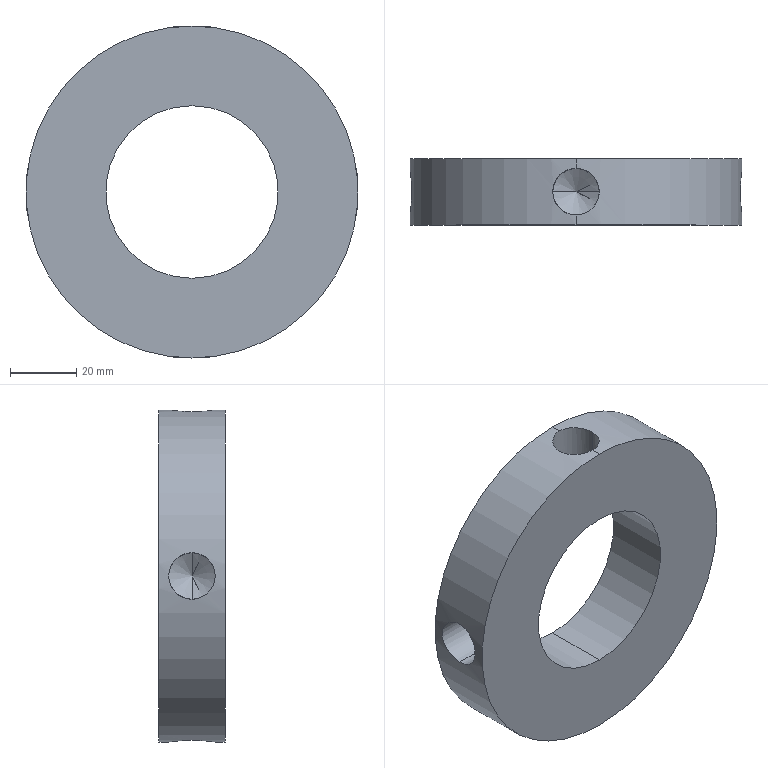Part | SolidWorks | features HoleWzd 2, 3DProfileFeature 1, CirPattern 1, Extrusion 1 | 1 solid | 22 faces | box 100 x 20 x 100 mm | volume 104092 mm3 | cylinder 12 | cone 8 | plane 2 | commonest cylinder face diameters 14 x8 52 x2 100 x2
STEP:
#1=CARTESIAN_POINT('',(-30.,10.,0.));
#2=VERTEX_POINT('',#1);
#3=CARTESIAN_POINT('',(-34.206,10.,7.));
#4=VERTEX_POINT('',#3);
#5=CARTESIAN_POINT('',(-34.206,10.,7.));
#6=DIRECTION('',(-0.515,0.,0.8572));
#7=VECTOR('',#6,1000.);
#8=LINE('',#5,#7);
#9=EDGE_CURVE('',#2,#4,#8,.T.);
#10=ORIENTED_EDGE('',*,*,#9,.F.);
#11=CARTESIAN_POINT('',(-34.206,10.,-7.));
#12=VERTEX_POINT('',#11);
#13=CARTESIAN_POINT('',(-34.206,10.,-7.));
#14=DIRECTION('',(-0.515,0.,-0.8572));
#15=VECTOR('',#14,1000.);
#16=LINE('',#13,#15);
#17=EDGE_CURVE('',#2,#12,#16,.T.);
#18=ORIENTED_EDGE('',*,*,#17,.T.);
#19=CARTESIAN_POINT('',(-34.206,10.,0.));
#20=DIRECTION('',(-1.,0.,0.));
#21=DIRECTION('',(0.,0.,1.));
#22=AXIS2_PLACEMENT_3D('',#19,#20,#21);
#23=CIRCLE('',#22,7.);
#24=EDGE_CURVE('',#12,#4,#23,.T.);
#25=ORIENTED_EDGE('',*,*,#24,.T.);
#26=EDGE_LOOP('',(#10,#18,#25));
#27=FACE_OUTER_BOUND('',#26,.T.);
#28=CARTESIAN_POINT('',(-34.206,10.,0.));
#29=DIRECTION('',(-1.,0.,0.));
#30=DIRECTION('',(0.,0.,1.));
#31=AXIS2_PLACEMENT_3D('',#28,#29,#30);
#32=CONICAL_SURFACE('',#31,7.,1.03);
#33=ADVANCED_FACE('',(#27),#32,.F.);
#34=ORIENTED_EDGE('',*,*,#24,.F.);
#35=CARTESIAN_POINT('',(-49.508,10.,-7.));
#36=VERTEX_POINT('',#35);
#37=CARTESIAN_POINT('',(-50.,10.,-7.));
#38=DIRECTION('',(-1.,0.,0.));
#39=VECTOR('',#38,1000.);
#40=LINE('',#37,#39);
#41=EDGE_CURVE('',#12,#36,#40,.T.);
#42=ORIENTED_EDGE('',*,*,#41,.T.);
#43=CARTESIAN_POINT('',(-49.508,10.,7.));
#44=VERTEX_POINT('',#43);
#45=CARTESIAN_POINT('',(-49.508,10.,7.));
#46=CARTESIAN_POINT('',(-49.508,9.537,7.));
#47=CARTESIAN_POINT('',(-49.514,9.082,6.954));
#48=CARTESIAN_POINT('',(-49.533,8.41,6.821));
#49=CARTESIAN_POINT('',(-49.54,8.188,6.765));
#50=CARTESIAN_POINT('',(-49.558,7.748,6.632));
#51=CARTESIAN_POINT('',(-49.569,7.529,6.554));
#52=CARTESIAN_POINT('',(-49.603,6.894,6.29));
#53=CARTESIAN_POINT('',(-49.63,6.492,6.075));
#54=CARTESIAN_POINT('',(-49.69,5.731,5.567));
#55=CARTESIAN_POINT('',(-49.722,5.372,5.271));
#56=CARTESIAN_POINT('',(-49.787,4.727,4.626));
#57=CARTESIAN_POINT('',(-49.818,4.437,4.274));
#58=CARTESIAN_POINT('',(-49.863,4.053,3.7));
#59=CARTESIAN_POINT('',(-49.878,3.935,3.502));
#60=CARTESIAN_POINT('',(-49.904,3.719,3.098));
#61=CARTESIAN_POINT('',(-49.929,3.524,2.686));
#62=CARTESIAN_POINT('',(-49.95,3.369,2.256));
#63=CARTESIAN_POINT('',(-49.967,3.236,1.817));
#64=CARTESIAN_POINT('',(-49.975,3.18,1.592));
#65=CARTESIAN_POINT('',(-49.994,3.045,0.9144));
#66=CARTESIAN_POINT('',(-50.,3.,0.4598));
#67=CARTESIAN_POINT('',(-50.,3.,-0.4546));
#68=CARTESIAN_POINT('',(-49.994,3.046,-0.9191));
#69=CARTESIAN_POINT('',(-49.969,3.225,-1.817));
#70=CARTESIAN_POINT('',(-49.951,3.357,-2.254));
#71=CARTESIAN_POINT('',(-49.917,3.62,-2.89));
#72=CARTESIAN_POINT('',(-49.904,3.72,-3.1));
#73=CARTESIAN_POINT('',(-49.877,3.936,-3.505));
#74=CARTESIAN_POINT('',(-49.863,4.054,-3.701));
#75=CARTESIAN_POINT('',(-49.819,4.434,-4.269));
#76=CARTESIAN_POINT('',(-49.787,4.724,-4.623));
#77=CARTESIAN_POINT('',(-49.722,5.376,-5.276));
#78=CARTESIAN_POINT('',(-49.69,5.729,-5.565));
#79=CARTESIAN_POINT('',(-49.645,6.298,-5.945));
#80=CARTESIAN_POINT('',(-49.631,6.493,-6.063));
#81=CARTESIAN_POINT('',(-49.604,6.899,-6.28));
#82=CARTESIAN_POINT('',(-49.592,7.108,-6.379));
#83=CARTESIAN_POINT('',(-49.557,7.744,-6.642));
#84=CARTESIAN_POINT('',(-49.539,8.18,-6.775));
#85=CARTESIAN_POINT('',(-49.514,9.078,-6.954));
#86=CARTESIAN_POINT('',(-49.508,9.543,-7.));
#87=CARTESIAN_POINT('',(-49.508,10.,-7.));
#88=B_SPLINE_CURVE_WITH_KNOTS('',3,(#45,#46,#47,#48,#49,#50,#51,#52,#53,#54,#55,#56,#57,#58,#59,#60,#61,#62,#63,#64,#65,#66,#67,#68,#69,#70,#71,#72,#73,#74,#75,#76,#77,#78,#79,#80,#81,#82,#83,#84,#85,#86,#87),.UNSPECIFIED.,.F.,.F.,(4,2,2,2,2,2,2,2,1,2,2,2,2,2,2,2,2,2,2,2,2,4),(0.,0.00137,0.002054,0.002739,0.004109,0.005478,0.006848,0.007532,0.008217,0.008902,0.009587,0.01096,0.01233,0.0137,0.01438,0.01506,0.01643,0.0178,0.01849,0.01917,0.02054,0.02191),.UNSPECIFIED.);
#89=EDGE_CURVE('',#44,#36,#88,.T.);
#90=ORIENTED_EDGE('',*,*,#89,.F.);
#91=CARTESIAN_POINT('',(-50.,10.,7.));
#92=DIRECTION('',(-1.,0.,0.));
#93=VECTOR('',#92,1000.);
#94=LINE('',#91,#93);
#95=EDGE_CURVE('',#4,#44,#94,.T.);
#96=ORIENTED_EDGE('',*,*,#95,.F.);
#97=EDGE_LOOP('',(#34,#42,#90,#96));
#98=FACE_OUTER_BOUND('',#97,.T.);
#99=CARTESIAN_POINT('',(-50.,10.,0.));
#100=DIRECTION('',(-1.,0.,0.));
#101=DIRECTION('',(0.,0.,1.));
#102=AXIS2_PLACEMENT_3D('',#99,#100,#101);
#103=CYLINDRICAL_SURFACE('',#102,7.);
#104=ADVANCED_FACE('',(#98),#103,.F.);
#105=CARTESIAN_POINT('',(0.,10.,-30.));
#106=VERTEX_POINT('',#105);
#107=CARTESIAN_POINT('',(-7.,10.,-34.206));
#108=VERTEX_POINT('',#107);
#109=CARTESIAN_POINT('',(-7.,10.,-34.206));
#110=DIRECTION('',(-0.8572,0.,-0.515));
#111=VECTOR('',#110,1000.);
#112=LINE('',#109,#111);
#113=EDGE_CURVE('',#106,#108,#112,.T.);
#114=ORIENTED_EDGE('',*,*,#113,.F.);
#115=CARTESIAN_POINT('',(7.,10.,-34.206));
#116=VERTEX_POINT('',#115);
#117=CARTESIAN_POINT('',(7.,10.,-34.206));
#118=DIRECTION('',(0.8572,0.,-0.515));
#119=VECTOR('',#118,1000.);
#120=LINE('',#117,#119);
#121=EDGE_CURVE('',#106,#116,#120,.T.);
#122=ORIENTED_EDGE('',*,*,#121,.T.);
#123=CARTESIAN_POINT('',(0.,10.,-34.206));
#124=DIRECTION('',(0.,0.,-1.));
#125=DIRECTION('',(-1.,0.,0.));
#126=AXIS2_PLACEMENT_3D('',#123,#124,#125);
#127=CIRCLE('',#126,7.);
#128=EDGE_CURVE('',#116,#108,#127,.T.);
#129=ORIENTED_EDGE('',*,*,#128,.T.);
#130=EDGE_LOOP('',(#114,#122,#129));
#131=FACE_OUTER_BOUND('',#130,.T.);
#132=CARTESIAN_POINT('',(0.,10.,-34.206));
#133=DIRECTION('',(0.,0.,-1.));
#134=DIRECTION('',(-1.,0.,0.));
#135=AXIS2_PLACEMENT_3D('',#132,#133,#134);
#136=CONICAL_SURFACE('',#135,7.,1.03);
#137=ADVANCED_FACE('',(#131),#136,.F.);
#138=ORIENTED_EDGE('',*,*,#128,.F.);
#139=CARTESIAN_POINT('',(7.,10.,-49.508));
#140=VERTEX_POINT('',#139);
#141=CARTESIAN_POINT('',(7.,10.,-50.));
#142=DIRECTION('',(0.,0.,-1.));
#143=VECTOR('',#142,1000.);
#144=LINE('',#141,#143);
#145=EDGE_CURVE('',#116,#140,#144,.T.);
#146=ORIENTED_EDGE('',*,*,#145,.T.);
#147=CARTESIAN_POINT('',(0.,3.,-50.));
#148=VERTEX_POINT('',#147);
#149=CARTESIAN_POINT('',(0.,3.,-50.));
#150=CARTESIAN_POINT('',(0.4572,3.,-50.));
#151=CARTESIAN_POINT('',(0.9121,3.044,-49.994));
#152=CARTESIAN_POINT('',(1.591,3.179,-49.975));
#153=CARTESIAN_POINT('',(1.815,3.236,-49.968));
#154=CARTESIAN_POINT('',(2.254,3.369,-49.95));
#155=CARTESIAN_POINT('',(2.684,3.523,-49.929));
#156=CARTESIAN_POINT('',(3.097,3.718,-49.904));
#157=CARTESIAN_POINT('',(3.501,3.934,-49.878));
#158=CARTESIAN_POINT('',(3.7,4.053,-49.863));
#159=CARTESIAN_POINT('',(4.273,4.437,-49.819));
#160=CARTESIAN_POINT('',(4.625,4.726,-49.787));
#161=CARTESIAN_POINT('',(5.271,5.371,-49.722));
#162=CARTESIAN_POINT('',(5.567,5.731,-49.69));
#163=CARTESIAN_POINT('',(6.074,6.491,-49.63));
#164=CARTESIAN_POINT('',(6.289,6.893,-49.603));
#165=CARTESIAN_POINT('',(6.553,7.529,-49.569));
#166=CARTESIAN_POINT('',(6.632,7.748,-49.558));
#167=CARTESIAN_POINT('',(6.765,8.188,-49.54));
#168=CARTESIAN_POINT('',(6.821,8.409,-49.533));
#169=CARTESIAN_POINT('',(6.954,9.081,-49.514));
#170=CARTESIAN_POINT('',(7.,9.537,-49.508));
#171=CARTESIAN_POINT('',(7.,10.,-49.508));
#172=B_SPLINE_CURVE_WITH_KNOTS('',3,(#149,#150,#151,#152,#153,#154,#155,#156,#157,#158,#159,#160,#161,#162,#163,#164,#165,#166,#167,#168,#169,#170,#171),.UNSPECIFIED.,.F.,.F.,(4,2,2,1,2,2,2,2,2,2,2,4),(0.02191,0.02328,0.02397,0.02465,0.02534,0.02602,0.02739,0.02876,0.03013,0.03082,0.0315,0.03287),.UNSPECIFIED.);
#173=EDGE_CURVE('',#148,#140,#172,.T.);
#174=ORIENTED_EDGE('',*,*,#173,.F.);
#175=CARTESIAN_POINT('',(-7.,10.,-49.508));
#176=VERTEX_POINT('',#175);
#177=CARTESIAN_POINT('',(-7.,10.,-49.508));
#178=CARTESIAN_POINT('',(-7.,9.543,-49.508));
#179=CARTESIAN_POINT('',(-6.954,9.079,-49.514));
#180=CARTESIAN_POINT('',(-6.775,8.181,-49.539));
#181=CARTESIAN_POINT('',(-6.642,7.744,-49.557));
#182=CARTESIAN_POINT('',(-6.379,7.108,-49.592));
#183=CARTESIAN_POINT('',(-6.28,6.898,-49.604));
#184=CARTESIAN_POINT('',(-6.063,6.494,-49.631));
#185=CARTESIAN_POINT('',(-5.945,6.298,-49.645));
#186=CARTESIAN_POINT('',(-5.565,5.73,-49.69));
#187=CARTESIAN_POINT('',(-5.275,5.376,-49.722));
#188=CARTESIAN_POINT('',(-4.623,4.723,-49.787));
#189=CARTESIAN_POINT('',(-4.27,4.434,-49.819));
#190=CARTESIAN_POINT('',(-3.702,4.054,-49.863));
#191=CARTESIAN_POINT('',(-3.506,3.937,-49.877));
#192=CARTESIAN_POINT('',(-3.101,3.72,-49.904));
#193=CARTESIAN_POINT('',(-2.891,3.621,-49.917));
#194=CARTESIAN_POINT('',(-2.256,3.358,-49.951));
#195=CARTESIAN_POINT('',(-1.819,3.225,-49.969));
#196=CARTESIAN_POINT('',(-0.9213,3.046,-49.994));
#197=CARTESIAN_POINT('',(-0.457,3.,-50.));
#198=CARTESIAN_POINT('',(0.,3.,-50.));
#199=B_SPLINE_CURVE_WITH_KNOTS('',3,(#177,#178,#179,#180,#181,#182,#183,#184,#185,#186,#187,#188,#189,#190,#191,#192,#193,#194,#195,#196,#197,#198),.UNSPECIFIED.,.F.,.F.,(4,2,2,2,2,2,2,2,2,2,4),(0.01096,0.01233,0.0137,0.01438,0.01507,0.01644,0.0178,0.01849,0.01917,0.02054,0.02191),.UNSPECIFIED.);
#200=EDGE_CURVE('',#176,#148,#199,.T.);
#201=ORIENTED_EDGE('',*,*,#200,.F.);
#202=CARTESIAN_POINT('',(-7.,10.,-50.));
#203=DIRECTION('',(0.,0.,-1.));
#204=VECTOR('',#203,1000.);
#205=LINE('',#202,#204);
#206=EDGE_CURVE('',#108,#176,#205,.T.);
#207=ORIENTED_EDGE('',*,*,#206,.F.);
#208=EDGE_LOOP('',(#138,#146,#174,#201,#207));
#209=FACE_OUTER_BOUND('',#208,.T.);
#210=CARTESIAN_POINT('',(0.,10.,-50.));
#211=DIRECTION('',(0.,0.,-1.));
#212=DIRECTION('',(-1.,0.,0.));
#213=AXIS2_PLACEMENT_3D('',#210,#211,#212);
#214=CYLINDRICAL_SURFACE('',#213,7.);
#215=ADVANCED_FACE('',(#209),#214,.F.);
#216=CARTESIAN_POINT('',(30.,10.,0.));
#217=VERTEX_POINT('',#216);
#218=CARTESIAN_POINT('',(34.206,10.,-7.));
#219=VERTEX_POINT('',#218);
#220=CARTESIAN_POINT('',(34.206,10.,-7.));
#221=DIRECTION('',(0.515,0.,-0.8572));
#222=VECTOR('',#221,1000.);
#223=LINE('',#220,#222);
#224=EDGE_CURVE('',#217,#219,#223,.T.);
#225=ORIENTED_EDGE('',*,*,#224,.F.);
#226=CARTESIAN_POINT('',(34.206,10.,7.));
#227=VERTEX_POINT('',#226);
#228=CARTESIAN_POINT('',(34.206,10.,7.));
#229=DIRECTION('',(0.515,0.,0.8572));
#230=VECTOR('',#229,1000.);
#231=LINE('',#228,#230);
#232=EDGE_CURVE('',#217,#227,#231,.T.);
#233=ORIENTED_EDGE('',*,*,#232,.T.);
#234=CARTESIAN_POINT('',(34.206,10.,0.));
#235=DIRECTION('',(1.,0.,0.));
#236=DIRECTION('',(0.,0.,-1.));
#237=AXIS2_PLACEMENT_3D('',#234,#235,#236);
#238=CIRCLE('',#237,7.);
#239=EDGE_CURVE('',#227,#219,#238,.T.);
#240=ORIENTED_EDGE('',*,*,#239,.T.);
#241=EDGE_LOOP('',(#225,#233,#240));
#242=FACE_OUTER_BOUND('',#241,.T.);
#243=CARTESIAN_POINT('',(34.206,10.,0.));
#244=DIRECTION('',(1.,0.,0.));
#245=DIRECTION('',(0.,0.,-1.));
#246=AXIS2_PLACEMENT_3D('',#243,#244,#245);
#247=CONICAL_SURFACE('',#246,7.,1.03);
#248=ADVANCED_FACE('',(#242),#247,.F.);
#249=ORIENTED_EDGE('',*,*,#239,.F.);
#250=CARTESIAN_POINT('',(49.508,10.,7.));
#251=VERTEX_POINT('',#250);
#252=CARTESIAN_POINT('',(50.,10.,7.));
#253=DIRECTION('',(1.,0.,0.));
#254=VECTOR('',#253,1000.);
#255=LINE('',#252,#254);
#256=EDGE_CURVE('',#227,#251,#255,.T.);
#257=ORIENTED_EDGE('',*,*,#256,.T.);
#258=CARTESIAN_POINT('',(49.508,10.,-7.));
#259=VERTEX_POINT('',#258);
#260=CARTESIAN_POINT('',(49.508,10.,-7.));
#261=CARTESIAN_POINT('',(49.508,9.537,-7.));
#262=CARTESIAN_POINT('',(49.514,9.082,-6.954));
#263=CARTESIAN_POINT('',(49.533,8.41,-6.821));
#264=CARTESIAN_POINT('',(49.54,8.188,-6.765));
#265=CARTESIAN_POINT('',(49.558,7.748,-6.632));
#266=CARTESIAN_POINT('',(49.569,7.529,-6.554));
#267=CARTESIAN_POINT('',(49.603,6.894,-6.29));
#268=CARTESIAN_POINT('',(49.63,6.492,-6.075));
#269=CARTESIAN_POINT('',(49.69,5.731,-5.567));
#270=CARTESIAN_POINT('',(49.722,5.372,-5.271));
#271=CARTESIAN_POINT('',(49.787,4.727,-4.626));
#272=CARTESIAN_POINT('',(49.818,4.437,-4.274));
#273=CARTESIAN_POINT('',(49.863,4.053,-3.7));
#274=CARTESIAN_POINT('',(49.878,3.935,-3.502));
#275=CARTESIAN_POINT('',(49.904,3.719,-3.098));
#276=CARTESIAN_POINT('',(49.929,3.524,-2.686));
#277=CARTESIAN_POINT('',(49.95,3.369,-2.256));
#278=CARTESIAN_POINT('',(49.967,3.236,-1.817));
#279=CARTESIAN_POINT('',(49.975,3.18,-1.592));
#280=CARTESIAN_POINT('',(49.994,3.045,-0.9144));
#281=CARTESIAN_POINT('',(50.,3.,-0.4598));
#282=CARTESIAN_POINT('',(50.,3.,0.4546));
#283=CARTESIAN_POINT('',(49.994,3.046,0.9191));
#284=CARTESIAN_POINT('',(49.969,3.225,1.817));
#285=CARTESIAN_POINT('',(49.951,3.357,2.254));
#286=CARTESIAN_POINT('',(49.917,3.62,2.89));
#287=CARTESIAN_POINT('',(49.904,3.72,3.1));
#288=CARTESIAN_POINT('',(49.877,3.936,3.505));
#289=CARTESIAN_POINT('',(49.863,4.054,3.701));
#290=CARTESIAN_POINT('',(49.819,4.434,4.269));
#291=CARTESIAN_POINT('',(49.787,4.724,4.623));
#292=CARTESIAN_POINT('',(49.722,5.376,5.276));
#293=CARTESIAN_POINT('',(49.69,5.729,5.565));
#294=CARTESIAN_POINT('',(49.645,6.298,5.945));
#295=CARTESIAN_POINT('',(49.631,6.493,6.063));
#296=CARTESIAN_POINT('',(49.604,6.899,6.28));
#297=CARTESIAN_POINT('',(49.592,7.108,6.379));
#298=CARTESIAN_POINT('',(49.557,7.744,6.642));
#299=CARTESIAN_POINT('',(49.539,8.18,6.775));
#300=CARTESIAN_POINT('',(49.514,9.078,6.954));
#301=CARTESIAN_POINT('',(49.508,9.543,7.));
#302=CARTESIAN_POINT('',(49.508,10.,7.));
#303=B_SPLINE_CURVE_WITH_KNOTS('',3,(#260,#261,#262,#263,#264,#265,#266,#267,#268,#269,#270,#271,#272,#273,#274,#275,#276,#277,#278,#279,#280,#281,#282,#283,#284,#285,#286,#287,#288,#289,#290,#291,#292,#293,#294,#295,#296,#297,#298,#299,#300,#301,#302),.UNSPECIFIED.,.F.,.F.,(4,2,2,2,2,2,2,2,1,2,2,2,2,2,2,2,2,2,2,2,2,4),(0.,0.00137,0.002054,0.002739,0.004109,0.005478,0.006848,0.007532,0.008217,0.008902,0.009587,0.01096,0.01233,0.0137,0.01438,0.01506,0.01643,0.0178,0.01849,0.01917,0.02054,0.02191),.UNSPECIFIED.);
#304=EDGE_CURVE('',#259,#251,#303,.T.);
#305=ORIENTED_EDGE('',*,*,#304,.F.);
#306=CARTESIAN_POINT('',(50.,10.,-7.));
#307=DIRECTION('',(1.,0.,0.));
#308=VECTOR('',#307,1000.);
#309=LINE('',#306,#308);
#310=EDGE_CURVE('',#219,#259,#309,.T.);
#311=ORIENTED_EDGE('',*,*,#310,.F.);
#312=EDGE_LOOP('',(#249,#257,#305,#311));
#313=FACE_OUTER_BOUND('',#312,.T.);
#314=CARTESIAN_POINT('',(50.,10.,0.));
#315=DIRECTION('',(1.,0.,0.));
#316=DIRECTION('',(0.,0.,-1.));
#317=AXIS2_PLACEMENT_3D('',#314,#315,#316);
#318=CYLINDRICAL_SURFACE('',#317,7.);
#319=ADVANCED_FACE('',(#313),#318,.F.);
#320=CARTESIAN_POINT('',(0.,10.,30.));
#321=VERTEX_POINT('',#320);
#322=CARTESIAN_POINT('',(7.,10.,34.206));
#323=VERTEX_POINT('',#322);
#324=CARTESIAN_POINT('',(7.,10.,34.206));
#325=DIRECTION('',(0.8572,0.,0.515));
#326=VECTOR('',#325,1000.);
#327=LINE('',#324,#326);
#328=EDGE_CURVE('',#321,#323,#327,.T.);
#329=ORIENTED_EDGE('',*,*,#328,.F.);
#330=CARTESIAN_POINT('',(-7.,10.,34.206));
#331=VERTEX_POINT('',#330);
#332=CARTESIAN_POINT('',(-7.,10.,34.206));
#333=DIRECTION('',(-0.8572,0.,0.515));
#334=VECTOR('',#333,1000.);
#335=LINE('',#332,#334);
#336=EDGE_CURVE('',#321,#331,#335,.T.);
#337=ORIENTED_EDGE('',*,*,#336,.T.);
#338=CARTESIAN_POINT('',(0.,10.,34.206));
#339=DIRECTION('',(0.,0.,1.));
#340=DIRECTION('',(1.,0.,0.));
#341=AXIS2_PLACEMENT_3D('',#338,#339,#340);
#342=CIRCLE('',#341,7.);
#343=EDGE_CURVE('',#331,#323,#342,.T.);
#344=ORIENTED_EDGE('',*,*,#343,.T.);
#345=EDGE_LOOP('',(#329,#337,#344));
#346=FACE_OUTER_BOUND('',#345,.T.);
#347=CARTESIAN_POINT('',(0.,10.,34.206));
#348=DIRECTION('',(0.,0.,1.));
#349=DIRECTION('',(1.,0.,0.));
#350=AXIS2_PLACEMENT_3D('',#347,#348,#349);
#351=CONICAL_SURFACE('',#350,7.,1.03);
#352=ADVANCED_FACE('',(#346),#351,.F.);
#353=ORIENTED_EDGE('',*,*,#343,.F.);
#354=CARTESIAN_POINT('',(-7.,10.,49.508));
#355=VERTEX_POINT('',#354);
#356=CARTESIAN_POINT('',(-7.,10.,50.));
#357=DIRECTION('',(0.,0.,1.));
#358=VECTOR('',#357,1000.);
#359=LINE('',#356,#358);
#360=EDGE_CURVE('',#331,#355,#359,.T.);
#361=ORIENTED_EDGE('',*,*,#360,.T.);
#362=CARTESIAN_POINT('',(0.,3.,50.));
#363=VERTEX_POINT('',#362);
#364=CARTESIAN_POINT('',(0.,3.,50.));
#365=CARTESIAN_POINT('',(-0.4571,3.,50.));
#366=CARTESIAN_POINT('',(-0.9214,3.046,49.994));
#367=CARTESIAN_POINT('',(-1.819,3.225,49.969));
#368=CARTESIAN_POINT('',(-2.256,3.358,49.951));
#369=CARTESIAN_POINT('',(-2.892,3.621,49.917));
#370=CARTESIAN_POINT('',(-3.102,3.72,49.904));
#371=CARTESIAN_POINT('',(-3.506,3.937,49.877));
#372=CARTESIAN_POINT('',(-3.702,4.055,49.863));
#373=CARTESIAN_POINT('',(-4.27,4.435,49.819));
#374=CARTESIAN_POINT('',(-4.624,4.725,49.787));
#375=CARTESIAN_POINT('',(-5.277,5.377,49.722));
#376=CARTESIAN_POINT('',(-5.566,5.73,49.69));
#377=CARTESIAN_POINT('',(-5.946,6.298,49.645));
#378=CARTESIAN_POINT('',(-6.063,6.494,49.631));
#379=CARTESIAN_POINT('',(-6.28,6.899,49.604));
#380=CARTESIAN_POINT('',(-6.379,7.109,49.591));
#381=CARTESIAN_POINT('',(-6.642,7.744,49.557));
#382=CARTESIAN_POINT('',(-6.775,8.181,49.539));
#383=CARTESIAN_POINT('',(-6.954,9.079,49.514));
#384=CARTESIAN_POINT('',(-7.,9.543,49.508));
#385=CARTESIAN_POINT('',(-7.,10.,49.508));
#386=B_SPLINE_CURVE_WITH_KNOTS('',3,(#364,#365,#366,#367,#368,#369,#370,#371,#372,#373,#374,#375,#376,#377,#378,#379,#380,#381,#382,#383,#384,#385),.UNSPECIFIED.,.F.,.F.,(4,2,2,2,2,2,2,2,2,2,4),(0.01096,0.01233,0.0137,0.01438,0.01507,0.01644,0.0178,0.01849,0.01917,0.02054,0.02191),.UNSPECIFIED.);
#387=EDGE_CURVE('',#363,#355,#386,.T.);
#388=ORIENTED_EDGE('',*,*,#387,.F.);
#389=CARTESIAN_POINT('',(7.,10.,49.508));
#390=VERTEX_POINT('',#389);
#391=CARTESIAN_POINT('',(7.,10.,49.508));
#392=CARTESIAN_POINT('',(7.,9.537,49.508));
#393=CARTESIAN_POINT('',(6.954,9.081,49.514));
#394=CARTESIAN_POINT('',(6.821,8.41,49.533));
#395=CARTESIAN_POINT('',(6.765,8.188,49.54));
#396=CARTESIAN_POINT('',(6.632,7.747,49.558));
#397=CARTESIAN_POINT('',(6.553,7.529,49.569));
#398=CARTESIAN_POINT('',(6.289,6.893,49.603));
#399=CARTESIAN_POINT('',(6.074,6.491,49.63));
#400=CARTESIAN_POINT('',(5.566,5.73,49.69));
#401=CARTESIAN_POINT('',(5.271,5.371,49.722));
#402=CARTESIAN_POINT('',(4.625,4.726,49.787));
#403=CARTESIAN_POINT('',(4.273,4.436,49.819));
#404=CARTESIAN_POINT('',(3.699,4.053,49.863));
#405=CARTESIAN_POINT('',(3.5,3.934,49.878));
#406=CARTESIAN_POINT('',(3.096,3.718,49.904));
#407=CARTESIAN_POINT('',(2.684,3.523,49.929));
#408=CARTESIAN_POINT('',(2.254,3.369,49.95));
#409=CARTESIAN_POINT('',(1.815,3.236,49.968));
#410=CARTESIAN_POINT('',(1.59,3.179,49.975));
#411=CARTESIAN_POINT('',(0.912,3.044,49.994));
#412=CARTESIAN_POINT('',(0.4573,3.,50.));
#413=CARTESIAN_POINT('',(0.,3.,50.));
#414=B_SPLINE_CURVE_WITH_KNOTS('',3,(#391,#392,#393,#394,#395,#396,#397,#398,#399,#400,#401,#402,#403,#404,#405,#406,#407,#408,#409,#410,#411,#412,#413),.UNSPECIFIED.,.F.,.F.,(4,2,2,2,2,2,2,2,1,2,2,4),(0.,0.00137,0.002055,0.00274,0.004109,0.005479,0.006849,0.007534,0.008219,0.008904,0.009589,0.01096),.UNSPECIFIED.);
#415=EDGE_CURVE('',#390,#363,#414,.T.);
#416=ORIENTED_EDGE('',*,*,#415,.F.);
#417=CARTESIAN_POINT('',(7.,10.,50.));
#418=DIRECTION('',(0.,0.,1.));
#419=VECTOR('',#418,1000.);
#420=LINE('',#417,#419);
#421=EDGE_CURVE('',#323,#390,#420,.T.);
#422=ORIENTED_EDGE('',*,*,#421,.F.);
#423=EDGE_LOOP('',(#353,#361,#388,#416,#422));
#424=FACE_OUTER_BOUND('',#423,.T.);
#425=CARTESIAN_POINT('',(0.,10.,50.));
#426=DIRECTION('',(0.,0.,1.));
#427=DIRECTION('',(1.,0.,0.));
#428=AXIS2_PLACEMENT_3D('',#425,#426,#427);
#429=CYLINDRICAL_SURFACE('',#428,7.);
#430=ADVANCED_FACE('',(#424),#429,.F.);
#431=CARTESIAN_POINT('',(0.,0.,-26.));
#432=VERTEX_POINT('',#431);
#433=CARTESIAN_POINT('',(0.,0.,26.));
#434=VERTEX_POINT('',#433);
#435=CARTESIAN_POINT('',(0.,0.,0.));
#436=DIRECTION('',(0.,1.,0.));
#437=DIRECTION('',(0.,0.,1.));
#438=AXIS2_PLACEMENT_3D('',#435,#436,#437);
#439=CIRCLE('',#438,26.);
#440=EDGE_CURVE('',#432,#434,#439,.T.);
#441=ORIENTED_EDGE('',*,*,#440,.F.);
#442=CARTESIAN_POINT('',(0.,20.,-26.));
#443=VERTEX_POINT('',#442);
#444=CARTESIAN_POINT('',(0.,20.,-26.));
#445=DIRECTION('',(0.,1.,0.));
#446=VECTOR('',#445,1000.);
#447=LINE('',#444,#446);
#448=EDGE_CURVE('',#432,#443,#447,.T.);
#449=ORIENTED_EDGE('',*,*,#448,.T.);
#450=CARTESIAN_POINT('',(0.,20.,26.));
#451=VERTEX_POINT('',#450);
#452=CARTESIAN_POINT('',(0.,20.,0.));
#453=DIRECTION('',(0.,1.,0.));
#454=DIRECTION('',(0.,0.,1.));
#455=AXIS2_PLACEMENT_3D('',#452,#453,#454);
#456=CIRCLE('',#455,26.);
#457=EDGE_CURVE('',#443,#451,#456,.T.);
#458=ORIENTED_EDGE('',*,*,#457,.T.);
#459=CARTESIAN_POINT('',(0.,20.,26.));
#460=DIRECTION('',(0.,1.,0.));
#461=VECTOR('',#460,1000.);
#462=LINE('',#459,#461);
#463=EDGE_CURVE('',#434,#451,#462,.T.);
#464=ORIENTED_EDGE('',*,*,#463,.F.);
#465=EDGE_LOOP('',(#441,#449,#458,#464));
#466=FACE_OUTER_BOUND('',#465,.T.);
#467=CARTESIAN_POINT('',(0.,20.,0.));
#468=DIRECTION('',(0.,1.,0.));
#469=DIRECTION('',(0.,0.,1.));
#470=AXIS2_PLACEMENT_3D('',#467,#468,#469);
#471=CYLINDRICAL_SURFACE('',#470,26.);
#472=ADVANCED_FACE('',(#466),#471,.F.);
#473=ORIENTED_EDGE('',*,*,#304,.T.);
#474=CARTESIAN_POINT('',(49.508,10.,7.));
#475=CARTESIAN_POINT('',(49.508,10.457,7.));
#476=CARTESIAN_POINT('',(49.514,10.912,6.956));
#477=CARTESIAN_POINT('',(49.533,11.59,6.821));
#478=CARTESIAN_POINT('',(49.54,11.815,6.765));
#479=CARTESIAN_POINT('',(49.558,12.253,6.631));
#480=CARTESIAN_POINT('',(49.579,12.683,6.478));
#481=CARTESIAN_POINT('',(49.604,13.095,6.283));
#482=CARTESIAN_POINT('',(49.631,13.5,6.067));
#483=CARTESIAN_POINT('',(49.645,13.698,5.948));
#484=CARTESIAN_POINT('',(49.69,14.272,5.565));
#485=CARTESIAN_POINT('',(49.722,14.624,5.275));
#486=CARTESIAN_POINT('',(49.786,15.269,4.631));
#487=CARTESIAN_POINT('',(49.819,15.565,4.271));
#488=CARTESIAN_POINT('',(49.878,16.073,3.512));
#489=CARTESIAN_POINT('',(49.905,16.288,3.11));
#490=CARTESIAN_POINT('',(49.939,16.552,2.474));
#491=CARTESIAN_POINT('',(49.95,16.631,2.256));
#492=CARTESIAN_POINT('',(49.967,16.764,1.816));
#493=CARTESIAN_POINT('',(49.975,16.82,1.594));
#494=CARTESIAN_POINT('',(49.993,16.954,0.9233));
#495=CARTESIAN_POINT('',(50.,17.,0.4674));
#496=CARTESIAN_POINT('',(50.,17.,-0.458));
#497=CARTESIAN_POINT('',(49.994,16.955,-0.913));
#498=CARTESIAN_POINT('',(49.975,16.822,-1.585));
#499=CARTESIAN_POINT('',(49.968,16.767,-1.807));
#500=CARTESIAN_POINT('',(49.95,16.633,-2.247));
#501=CARTESIAN_POINT('',(49.94,16.555,-2.466));
#502=CARTESIAN_POINT('',(49.906,16.292,-3.101));
#503=CARTESIAN_POINT('',(49.879,16.078,-3.503));
#504=CARTESIAN_POINT('',(49.834,15.697,-4.074));
#505=CARTESIAN_POINT('',(49.819,15.559,-4.26));
#506=CARTESIAN_POINT('',(49.787,15.268,-4.616));
#507=CARTESIAN_POINT('',(49.771,15.114,-4.785));
#508=CARTESIAN_POINT('',(49.723,14.631,-5.269));
#509=CARTESIAN_POINT('',(49.691,14.279,-5.559));
#510=CARTESIAN_POINT('',(49.646,13.705,-5.943));
#511=CARTESIAN_POINT('',(49.631,13.507,-6.062));
#512=CARTESIAN_POINT('',(49.604,13.104,-6.278));
#513=CARTESIAN_POINT('',(49.579,12.692,-6.474));
#514=CARTESIAN_POINT('',(49.559,12.262,-6.628));
#515=CARTESIAN_POINT('',(49.541,11.824,-6.762));
#516=CARTESIAN_POINT('',(49.533,11.599,-6.819));
#517=CARTESIAN_POINT('',(49.514,10.921,-6.955));
#518=CARTESIAN_POINT('',(49.508,10.463,-7.));
#519=CARTESIAN_POINT('',(49.508,10.,-7.));
#520=B_SPLINE_CURVE_WITH_KNOTS('',3,(#474,#475,#476,#477,#478,#479,#480,#481,#482,#483,#484,#485,#486,#487,#488,#489,#490,#491,#492,#493,#494,#495,#496,#497,#498,#499,#500,#501,#502,#503,#504,#505,#506,#507,#508,#509,#510,#511,#512,#513,#514,#515,#516,#517,#518,#519),.UNSPECIFIED.,.F.,.F.,(4,2,2,1,2,2,2,2,2,2,2,2,2,2,2,2,2,2,2,2,1,2,2,4),(0.02191,0.02328,0.02397,0.02465,0.02534,0.02602,0.02739,0.02876,0.03013,0.03081,0.0315,0.03287,0.03423,0.03492,0.0356,0.03697,0.03766,0.03834,0.03971,0.0404,0.04108,0.04177,0.04245,0.04382),.UNSPECIFIED.);
#521=EDGE_CURVE('',#251,#259,#520,.T.);
#522=ORIENTED_EDGE('',*,*,#521,.T.);
#523=EDGE_LOOP('',(#473,#522));
#524=FACE_BOUND('',#523,.T.);
#525=CARTESIAN_POINT('',(0.,20.,50.));
#526=VERTEX_POINT('',#525);
#527=CARTESIAN_POINT('',(0.,20.,-50.));
#528=VERTEX_POINT('',#527);
#529=CARTESIAN_POINT('',(0.,20.,0.));
#530=DIRECTION('',(0.,1.,0.));
#531=DIRECTION('',(0.,0.,1.));
#532=AXIS2_PLACEMENT_3D('',#529,#530,#531);
#533=CIRCLE('',#532,50.);
#534=EDGE_CURVE('',#526,#528,#533,.T.);
#535=ORIENTED_EDGE('',*,*,#534,.F.);
#536=CARTESIAN_POINT('',(0.,17.,50.));
#537=VERTEX_POINT('',#536);
#538=CARTESIAN_POINT('',(0.,20.,50.));
#539=DIRECTION('',(0.,-1.,0.));
#540=VECTOR('',#539,1000.);
#541=LINE('',#538,#540);
#542=EDGE_CURVE('',#526,#537,#541,.T.);
#543=ORIENTED_EDGE('',*,*,#542,.T.);
#544=CARTESIAN_POINT('',(0.,17.,50.));
#545=CARTESIAN_POINT('',(0.4624,17.,50.));
#546=CARTESIAN_POINT('',(0.9173,16.955,49.994));
#547=CARTESIAN_POINT('',(1.589,16.821,49.975));
#548=CARTESIAN_POINT('',(1.811,16.766,49.968));
#549=CARTESIAN_POINT('',(2.251,16.632,49.95));
#550=CARTESIAN_POINT('',(2.469,16.554,49.939));
#551=CARTESIAN_POINT('',(3.104,16.291,49.905));
#552=CARTESIAN_POINT('',(3.506,16.076,49.878));
#553=CARTESIAN_POINT('',(4.076,15.695,49.834));
#554=CARTESIAN_POINT('',(4.262,15.558,49.818));
#555=CARTESIAN_POINT('',(4.618,15.266,49.787));
#556=CARTESIAN_POINT('',(4.787,15.112,49.771));
#557=CARTESIAN_POINT('',(5.27,14.629,49.723));
#558=CARTESIAN_POINT('',(5.56,14.278,49.691));
#559=CARTESIAN_POINT('',(5.944,13.704,49.646));
#560=CARTESIAN_POINT('',(6.063,13.506,49.631));
#561=CARTESIAN_POINT('',(6.279,13.103,49.604));
#562=CARTESIAN_POINT('',(6.474,12.691,49.579));
#563=CARTESIAN_POINT('',(6.629,12.261,49.559));
#564=CARTESIAN_POINT('',(6.762,11.823,49.541));
#565=CARTESIAN_POINT('',(6.819,11.598,49.533));
#566=CARTESIAN_POINT('',(6.955,10.92,49.514));
#567=CARTESIAN_POINT('',(7.,10.463,49.508));
#568=CARTESIAN_POINT('',(7.,10.,49.508));
#569=B_SPLINE_CURVE_WITH_KNOTS('',3,(#544,#545,#546,#547,#548,#549,#550,#551,#552,#553,#554,#555,#556,#557,#558,#559,#560,#561,#562,#563,#564,#565,#566,#567,#568),.UNSPECIFIED.,.F.,.F.,(4,2,2,2,2,2,2,2,2,1,2,2,4),(0.03287,0.03424,0.03492,0.03561,0.03698,0.03766,0.03834,0.03971,0.0404,0.04108,0.04177,0.04245,0.04382),.UNSPECIFIED.);
#570=EDGE_CURVE('',#537,#390,#569,.T.);
#571=ORIENTED_EDGE('',*,*,#570,.T.);
#572=ORIENTED_EDGE('',*,*,#415,.T.);
#573=CARTESIAN_POINT('',(0.,0.,50.));
#574=VERTEX_POINT('',#573);
#575=CARTESIAN_POINT('',(0.,20.,50.));
#576=DIRECTION('',(0.,-1.,0.));
#577=VECTOR('',#576,1000.);
#578=LINE('',#575,#577);
#579=EDGE_CURVE('',#363,#574,#578,.T.);
#580=ORIENTED_EDGE('',*,*,#579,.T.);
#581=CARTESIAN_POINT('',(0.,0.,-50.));
#582=VERTEX_POINT('',#581);
#583=CARTESIAN_POINT('',(0.,0.,0.));
#584=DIRECTION('',(0.,1.,0.));
#585=DIRECTION('',(0.,0.,1.));
#586=AXIS2_PLACEMENT_3D('',#583,#584,#585);
#587=CIRCLE('',#586,50.);
#588=EDGE_CURVE('',#574,#582,#587,.T.);
#589=ORIENTED_EDGE('',*,*,#588,.T.);
#590=CARTESIAN_POINT('',(0.,20.,-50.));
#591=DIRECTION('',(0.,-1.,0.));
#592=VECTOR('',#591,1000.);
#593=LINE('',#590,#592);
#594=EDGE_CURVE('',#148,#582,#593,.T.);
#595=ORIENTED_EDGE('',*,*,#594,.F.);
#596=ORIENTED_EDGE('',*,*,#173,.T.);
#597=CARTESIAN_POINT('',(0.,17.,-50.));
#598=VERTEX_POINT('',#597);
#599=CARTESIAN_POINT('',(7.,10.,-49.508));
#600=CARTESIAN_POINT('',(7.,10.462,-49.508));
#601=CARTESIAN_POINT('',(6.955,10.917,-49.514));
#602=CARTESIAN_POINT('',(6.821,11.589,-49.533));
#603=CARTESIAN_POINT('',(6.766,11.811,-49.54));
#604=CARTESIAN_POINT('',(6.632,12.251,-49.558));
#605=CARTESIAN_POINT('',(6.554,12.469,-49.569));
#606=CARTESIAN_POINT('',(6.291,13.104,-49.603));
#607=CARTESIAN_POINT('',(6.076,13.506,-49.63));
#608=CARTESIAN_POINT('',(5.695,14.076,-49.675));
#609=CARTESIAN_POINT('',(5.558,14.262,-49.69));
#610=CARTESIAN_POINT('',(5.266,14.618,-49.722));
#611=CARTESIAN_POINT('',(5.113,14.787,-49.738));
#612=CARTESIAN_POINT('',(4.629,15.27,-49.786));
#613=CARTESIAN_POINT('',(4.278,15.56,-49.818));
#614=CARTESIAN_POINT('',(3.704,15.944,-49.863));
#615=CARTESIAN_POINT('',(3.506,16.063,-49.877));
#616=CARTESIAN_POINT('',(3.103,16.279,-49.904));
#617=CARTESIAN_POINT('',(2.691,16.474,-49.929));
#618=CARTESIAN_POINT('',(2.261,16.629,-49.949));
#619=CARTESIAN_POINT('',(1.823,16.762,-49.967));
#620=CARTESIAN_POINT('',(1.598,16.819,-49.975));
#621=CARTESIAN_POINT('',(0.9202,16.955,-49.994));
#622=CARTESIAN_POINT('',(0.4628,17.,-50.));
#623=CARTESIAN_POINT('',(0.,17.,-50.));
#624=B_SPLINE_CURVE_WITH_KNOTS('',3,(#599,#600,#601,#602,#603,#604,#605,#606,#607,#608,#609,#610,#611,#612,#613,#614,#615,#616,#617,#618,#619,#620,#621,#622,#623),.UNSPECIFIED.,.F.,.F.,(4,2,2,2,2,2,2,2,2,1,2,2,4),(0.03287,0.03424,0.03492,0.03561,0.03698,0.03766,0.03834,0.03971,0.0404,0.04108,0.04177,0.04245,0.04382),.UNSPECIFIED.);
#625=EDGE_CURVE('',#140,#598,#624,.T.);
#626=ORIENTED_EDGE('',*,*,#625,.T.);
#627=CARTESIAN_POINT('',(0.,20.,-50.));
#628=DIRECTION('',(0.,-1.,0.));
#629=VECTOR('',#628,1000.);
#630=LINE('',#627,#629);
#631=EDGE_CURVE('',#528,#598,#630,.T.);
#632=ORIENTED_EDGE('',*,*,#631,.F.);
#633=EDGE_LOOP('',(#535,#543,#571,#572,#580,#589,#595,#596,#626,#632));
#634=FACE_OUTER_BOUND('',#633,.T.);
#635=CARTESIAN_POINT('',(0.,20.,0.));
#636=DIRECTION('',(0.,-1.,0.));
#637=DIRECTION('',(0.,0.,-1.));
#638=AXIS2_PLACEMENT_3D('',#635,#636,#637);
#639=CYLINDRICAL_SURFACE('',#638,50.);
#640=ADVANCED_FACE('',(#524,#634),#639,.T.);
#641=ORIENTED_EDGE('',*,*,#542,.F.);
#642=CARTESIAN_POINT('',(0.,20.,0.));
#643=DIRECTION('',(0.,1.,0.));
#644=DIRECTION('',(0.,0.,1.));
#645=AXIS2_PLACEMENT_3D('',#642,#643,#644);
#646=CIRCLE('',#645,50.);
#647=EDGE_CURVE('',#528,#526,#646,.T.);
#648=ORIENTED_EDGE('',*,*,#647,.F.);
#649=ORIENTED_EDGE('',*,*,#631,.T.);
#650=CARTESIAN_POINT('',(0.,17.,-50.));
#651=CARTESIAN_POINT('',(-0.4632,17.,-50.));
#652=CARTESIAN_POINT('',(-0.9186,16.954,-49.994));
#653=CARTESIAN_POINT('',(-1.59,16.821,-49.975));
#654=CARTESIAN_POINT('',(-1.812,16.765,-49.968));
#655=CARTESIAN_POINT('',(-2.253,16.632,-49.95));
#656=CARTESIAN_POINT('',(-2.471,16.553,-49.939));
#657=CARTESIAN_POINT('',(-3.107,16.289,-49.905));
#658=CARTESIAN_POINT('',(-3.509,16.074,-49.878));
#659=CARTESIAN_POINT('',(-4.27,15.566,-49.819));
#660=CARTESIAN_POINT('',(-4.629,15.27,-49.786));
#661=CARTESIAN_POINT('',(-5.274,14.625,-49.722));
#662=CARTESIAN_POINT('',(-5.564,14.273,-49.69));
#663=CARTESIAN_POINT('',(-5.947,13.699,-49.645));
#664=CARTESIAN_POINT('',(-6.066,13.5,-49.631));
#665=CARTESIAN_POINT('',(-6.282,13.096,-49.604));
#666=CARTESIAN_POINT('',(-6.477,12.684,-49.579));
#667=CARTESIAN_POINT('',(-6.631,12.254,-49.558));
#668=CARTESIAN_POINT('',(-6.764,11.815,-49.54));
#669=CARTESIAN_POINT('',(-6.821,11.59,-49.533));
#670=CARTESIAN_POINT('',(-6.956,10.912,-49.514));
#671=CARTESIAN_POINT('',(-7.,10.457,-49.508));
#672=CARTESIAN_POINT('',(-7.,10.,-49.508));
#673=B_SPLINE_CURVE_WITH_KNOTS('',3,(#650,#651,#652,#653,#654,#655,#656,#657,#658,#659,#660,#661,#662,#663,#664,#665,#666,#667,#668,#669,#670,#671,#672),.UNSPECIFIED.,.F.,.F.,(4,2,2,2,2,2,2,2,1,2,2,4),(0.,0.00137,0.002055,0.00274,0.004109,0.005479,0.006849,0.007534,0.008219,0.008904,0.009589,0.01096),.UNSPECIFIED.);
#674=EDGE_CURVE('',#598,#176,#673,.T.);
#675=ORIENTED_EDGE('',*,*,#674,.T.);
#676=ORIENTED_EDGE('',*,*,#200,.T.);
#677=ORIENTED_EDGE('',*,*,#594,.T.);
#678=CARTESIAN_POINT('',(0.,0.,0.));
#679=DIRECTION('',(0.,1.,0.));
#680=DIRECTION('',(0.,0.,1.));
#681=AXIS2_PLACEMENT_3D('',#678,#679,#680);
#682=CIRCLE('',#681,50.);
#683=EDGE_CURVE('',#582,#574,#682,.T.);
#684=ORIENTED_EDGE('',*,*,#683,.T.);
#685=ORIENTED_EDGE('',*,*,#579,.F.);
#686=ORIENTED_EDGE('',*,*,#387,.T.);
#687=CARTESIAN_POINT('',(-7.,10.,49.508));
#688=CARTESIAN_POINT('',(-7.,10.457,49.508));
#689=CARTESIAN_POINT('',(-6.956,10.912,49.514));
#690=CARTESIAN_POINT('',(-6.821,11.591,49.533));
#691=CARTESIAN_POINT('',(-6.764,11.815,49.54));
#692=CARTESIAN_POINT('',(-6.631,12.254,49.558));
#693=CARTESIAN_POINT('',(-6.477,12.684,49.579));
#694=CARTESIAN_POINT('',(-6.282,13.097,49.604));
#695=CARTESIAN_POINT('',(-6.066,13.501,49.631));
#696=CARTESIAN_POINT('',(-5.947,13.7,49.645));
#697=CARTESIAN_POINT('',(-5.563,14.273,49.69));
#698=CARTESIAN_POINT('',(-5.274,14.625,49.722));
#699=CARTESIAN_POINT('',(-4.629,15.271,49.786));
#700=CARTESIAN_POINT('',(-4.269,15.567,49.819));
#701=CARTESIAN_POINT('',(-3.509,16.074,49.878));
#702=CARTESIAN_POINT('',(-3.107,16.289,49.905));
#703=CARTESIAN_POINT('',(-2.471,16.553,49.939));
#704=CARTESIAN_POINT('',(-2.252,16.632,49.95));
#705=CARTESIAN_POINT('',(-1.812,16.765,49.968));
#706=CARTESIAN_POINT('',(-1.591,16.821,49.975));
#707=CARTESIAN_POINT('',(-0.919,16.954,49.994));
#708=CARTESIAN_POINT('',(-0.4628,17.,50.));
#709=CARTESIAN_POINT('',(0.,17.,50.));
#710=B_SPLINE_CURVE_WITH_KNOTS('',3,(#687,#688,#689,#690,#691,#692,#693,#694,#695,#696,#697,#698,#699,#700,#701,#702,#703,#704,#705,#706,#707,#708,#709),.UNSPECIFIED.,.F.,.F.,(4,2,2,1,2,2,2,2,2,2,2,4),(0.02191,0.02328,0.02397,0.02465,0.02534,0.02602,0.02739,0.02876,0.03013,0.03082,0.0315,0.03287),.UNSPECIFIED.);
#711=EDGE_CURVE('',#355,#537,#710,.T.);
#712=ORIENTED_EDGE('',*,*,#711,.T.);
#713=EDGE_LOOP('',(#641,#648,#649,#675,#676,#677,#684,#685,#686,#712));
#714=FACE_OUTER_BOUND('',#713,.T.);
#715=ORIENTED_EDGE('',*,*,#89,.T.);
#716=CARTESIAN_POINT('',(-49.508,10.,-7.));
#717=CARTESIAN_POINT('',(-49.508,10.457,-7.));
#718=CARTESIAN_POINT('',(-49.514,10.912,-6.956));
#719=CARTESIAN_POINT('',(-49.533,11.59,-6.821));
#720=CARTESIAN_POINT('',(-49.54,11.815,-6.765));
#721=CARTESIAN_POINT('',(-49.558,12.253,-6.631));
#722=CARTESIAN_POINT('',(-49.579,12.683,-6.478));
#723=CARTESIAN_POINT('',(-49.604,13.095,-6.283));
#724=CARTESIAN_POINT('',(-49.631,13.5,-6.067));
#725=CARTESIAN_POINT('',(-49.645,13.698,-5.948));
#726=CARTESIAN_POINT('',(-49.69,14.272,-5.565));
#727=CARTESIAN_POINT('',(-49.722,14.624,-5.275));
#728=CARTESIAN_POINT('',(-49.786,15.269,-4.631));
#729=CARTESIAN_POINT('',(-49.819,15.565,-4.271));
#730=CARTESIAN_POINT('',(-49.878,16.073,-3.512));
#731=CARTESIAN_POINT('',(-49.905,16.288,-3.11));
#732=CARTESIAN_POINT('',(-49.939,16.552,-2.474));
#733=CARTESIAN_POINT('',(-49.95,16.631,-2.256));
#734=CARTESIAN_POINT('',(-49.967,16.764,-1.816));
#735=CARTESIAN_POINT('',(-49.975,16.82,-1.594));
#736=CARTESIAN_POINT('',(-49.993,16.954,-0.9233));
#737=CARTESIAN_POINT('',(-50.,17.,-0.4674));
#738=CARTESIAN_POINT('',(-50.,17.,0.458));
#739=CARTESIAN_POINT('',(-49.994,16.955,0.913));
#740=CARTESIAN_POINT('',(-49.975,16.822,1.585));
#741=CARTESIAN_POINT('',(-49.968,16.767,1.807));
#742=CARTESIAN_POINT('',(-49.95,16.633,2.247));
#743=CARTESIAN_POINT('',(-49.94,16.555,2.466));
#744=CARTESIAN_POINT('',(-49.906,16.292,3.101));
#745=CARTESIAN_POINT('',(-49.879,16.078,3.503));
#746=CARTESIAN_POINT('',(-49.834,15.697,4.074));
#747=CARTESIAN_POINT('',(-49.819,15.559,4.26));
#748=CARTESIAN_POINT('',(-49.787,15.268,4.616));
#749=CARTESIAN_POINT('',(-49.771,15.114,4.785));
#750=CARTESIAN_POINT('',(-49.723,14.631,5.269));
#751=CARTESIAN_POINT('',(-49.691,14.279,5.559));
#752=CARTESIAN_POINT('',(-49.646,13.705,5.943));
#753=CARTESIAN_POINT('',(-49.631,13.507,6.062));
#754=CARTESIAN_POINT('',(-49.604,13.104,6.278));
#755=CARTESIAN_POINT('',(-49.579,12.692,6.474));
#756=CARTESIAN_POINT('',(-49.559,12.262,6.628));
#757=CARTESIAN_POINT('',(-49.541,11.824,6.762));
#758=CARTESIAN_POINT('',(-49.533,11.599,6.819));
#759=CARTESIAN_POINT('',(-49.514,10.921,6.955));
#760=CARTESIAN_POINT('',(-49.508,10.463,7.));
#761=CARTESIAN_POINT('',(-49.508,10.,7.));
#762=B_SPLINE_CURVE_WITH_KNOTS('',3,(#716,#717,#718,#719,#720,#721,#722,#723,#724,#725,#726,#727,#728,#729,#730,#731,#732,#733,#734,#735,#736,#737,#738,#739,#740,#741,#742,#743,#744,#745,#746,#747,#748,#749,#750,#751,#752,#753,#754,#755,#756,#757,#758,#759,#760,#761),.UNSPECIFIED.,.F.,.F.,(4,2,2,1,2,2,2,2,2,2,2,2,2,2,2,2,2,2,2,2,1,2,2,4),(0.02191,0.02328,0.02397,0.02465,0.02534,0.02602,0.02739,0.02876,0.03013,0.03081,0.0315,0.03287,0.03423,0.03492,0.0356,0.03697,0.03766,0.03834,0.03971,0.0404,0.04108,0.04177,0.04245,0.04382),.UNSPECIFIED.);
#763=EDGE_CURVE('',#36,#44,#762,.T.);
#764=ORIENTED_EDGE('',*,*,#763,.T.);
#765=EDGE_LOOP('',(#715,#764));
#766=FACE_BOUND('',#765,.T.);
#767=CARTESIAN_POINT('',(0.,20.,0.));
#768=DIRECTION('',(0.,-1.,0.));
#769=DIRECTION('',(0.,0.,-1.));
#770=AXIS2_PLACEMENT_3D('',#767,#768,#769);
#771=CYLINDRICAL_SURFACE('',#770,50.);
#772=ADVANCED_FACE('',(#714,#766),#771,.T.);
#773=CARTESIAN_POINT('',(0.,20.,0.));
#774=DIRECTION('',(0.,1.,0.));
#775=DIRECTION('',(0.,0.,1.));
#776=AXIS2_PLACEMENT_3D('',#773,#774,#775);
#777=CIRCLE('',#776,26.);
#778=EDGE_CURVE('',#451,#443,#777,.T.);
#779=ORIENTED_EDGE('',*,*,#778,.F.);
#780=ORIENTED_EDGE('',*,*,#457,.F.);
#781=EDGE_LOOP('',(#779,#780));
#782=FACE_BOUND('',#781,.T.);
#783=ORIENTED_EDGE('',*,*,#647,.T.);
#784=ORIENTED_EDGE('',*,*,#534,.T.);
#785=EDGE_LOOP('',(#783,#784));
#786=FACE_OUTER_BOUND('',#785,.T.);
#787=CARTESIAN_POINT('',(0.,20.,0.));
#788=DIRECTION('',(0.,1.,0.));
#789=DIRECTION('',(0.,0.,1.));
#790=AXIS2_PLACEMENT_3D('',#787,#788,#789);
#791=PLANE('',#790);
#792=ADVANCED_FACE('',(#782,#786),#791,.T.);
#793=CARTESIAN_POINT('',(0.,0.,0.));
#794=DIRECTION('',(0.,1.,0.));
#795=DIRECTION('',(0.,0.,1.));
#796=AXIS2_PLACEMENT_3D('',#793,#794,#795);
#797=CIRCLE('',#796,26.);
#798=EDGE_CURVE('',#434,#432,#797,.T.);
#799=ORIENTED_EDGE('',*,*,#798,.T.);
#800=ORIENTED_EDGE('',*,*,#440,.T.);
#801=EDGE_LOOP('',(#799,#800));
#802=FACE_BOUND('',#801,.T.);
#803=ORIENTED_EDGE('',*,*,#683,.F.);
#804=ORIENTED_EDGE('',*,*,#588,.F.);
#805=EDGE_LOOP('',(#803,#804));
#806=FACE_OUTER_BOUND('',#805,.T.);
#807=CARTESIAN_POINT('',(0.,0.,0.));
#808=DIRECTION('',(0.,1.,0.));
#809=DIRECTION('',(0.,0.,1.));
#810=AXIS2_PLACEMENT_3D('',#807,#808,#809);
#811=PLANE('',#810);
#812=ADVANCED_FACE('',(#802,#806),#811,.F.);
#813=ORIENTED_EDGE('',*,*,#448,.F.);
#814=ORIENTED_EDGE('',*,*,#798,.F.);
#815=ORIENTED_EDGE('',*,*,#463,.T.);
#816=ORIENTED_EDGE('',*,*,#778,.T.);
#817=EDGE_LOOP('',(#813,#814,#815,#816));
#818=FACE_OUTER_BOUND('',#817,.T.);
#819=CARTESIAN_POINT('',(0.,20.,0.));
#820=DIRECTION('',(0.,1.,0.));
#821=DIRECTION('',(0.,0.,1.));
#822=AXIS2_PLACEMENT_3D('',#819,#820,#821);
#823=CYLINDRICAL_SURFACE('',#822,26.);
#824=ADVANCED_FACE('',(#818),#823,.F.);
#825=ORIENTED_EDGE('',*,*,#360,.F.);
#826=CARTESIAN_POINT('',(0.,10.,34.206));
#827=DIRECTION('',(0.,0.,1.));
#828=DIRECTION('',(1.,0.,0.));
#829=AXIS2_PLACEMENT_3D('',#826,#827,#828);
#830=CIRCLE('',#829,7.);
#831=EDGE_CURVE('',#323,#331,#830,.T.);
#832=ORIENTED_EDGE('',*,*,#831,.F.);
#833=ORIENTED_EDGE('',*,*,#421,.T.);
#834=ORIENTED_EDGE('',*,*,#570,.F.);
#835=ORIENTED_EDGE('',*,*,#711,.F.);
#836=EDGE_LOOP('',(#825,#832,#833,#834,#835));
#837=FACE_OUTER_BOUND('',#836,.T.);
#838=CARTESIAN_POINT('',(0.,10.,50.));
#839=DIRECTION('',(0.,0.,1.));
#840=DIRECTION('',(1.,0.,0.));
#841=AXIS2_PLACEMENT_3D('',#838,#839,#840);
#842=CYLINDRICAL_SURFACE('',#841,7.);
#843=ADVANCED_FACE('',(#837),#842,.F.);
#844=ORIENTED_EDGE('',*,*,#336,.F.);
#845=ORIENTED_EDGE('',*,*,#328,.T.);
#846=ORIENTED_EDGE('',*,*,#831,.T.);
#847=EDGE_LOOP('',(#844,#845,#846));
#848=FACE_OUTER_BOUND('',#847,.T.);
#849=CARTESIAN_POINT('',(0.,10.,34.206));
#850=DIRECTION('',(0.,0.,1.));
#851=DIRECTION('',(1.,0.,0.));
#852=AXIS2_PLACEMENT_3D('',#849,#850,#851);
#853=CONICAL_SURFACE('',#852,7.,1.03);
#854=ADVANCED_FACE('',(#848),#853,.F.);
#855=ORIENTED_EDGE('',*,*,#256,.F.);
#856=CARTESIAN_POINT('',(34.206,10.,0.));
#857=DIRECTION('',(1.,0.,0.));
#858=DIRECTION('',(0.,0.,-1.));
#859=AXIS2_PLACEMENT_3D('',#856,#857,#858);
#860=CIRCLE('',#859,7.);
#861=EDGE_CURVE('',#219,#227,#860,.T.);
#862=ORIENTED_EDGE('',*,*,#861,.F.);
#863=ORIENTED_EDGE('',*,*,#310,.T.);
#864=ORIENTED_EDGE('',*,*,#521,.F.);
#865=EDGE_LOOP('',(#855,#862,#863,#864));
#866=FACE_OUTER_BOUND('',#865,.T.);
#867=CARTESIAN_POINT('',(50.,10.,0.));
#868=DIRECTION('',(1.,0.,0.));
#869=DIRECTION('',(0.,0.,-1.));
#870=AXIS2_PLACEMENT_3D('',#867,#868,#869);
#871=CYLINDRICAL_SURFACE('',#870,7.);
#872=ADVANCED_FACE('',(#866),#871,.F.);
#873=ORIENTED_EDGE('',*,*,#232,.F.);
#874=ORIENTED_EDGE('',*,*,#224,.T.);
#875=ORIENTED_EDGE('',*,*,#861,.T.);
#876=EDGE_LOOP('',(#873,#874,#875));
#877=FACE_OUTER_BOUND('',#876,.T.);
#878=CARTESIAN_POINT('',(34.206,10.,0.));
#879=DIRECTION('',(1.,0.,0.));
#880=DIRECTION('',(0.,0.,-1.));
#881=AXIS2_PLACEMENT_3D('',#878,#879,#880);
#882=CONICAL_SURFACE('',#881,7.,1.03);
#883=ADVANCED_FACE('',(#877),#882,.F.);
#884=ORIENTED_EDGE('',*,*,#145,.F.);
#885=CARTESIAN_POINT('',(0.,10.,-34.206));
#886=DIRECTION('',(0.,0.,-1.));
#887=DIRECTION('',(-1.,0.,0.));
#888=AXIS2_PLACEMENT_3D('',#885,#886,#887);
#889=CIRCLE('',#888,7.);
#890=EDGE_CURVE('',#108,#116,#889,.T.);
#891=ORIENTED_EDGE('',*,*,#890,.F.);
#892=ORIENTED_EDGE('',*,*,#206,.T.);
#893=ORIENTED_EDGE('',*,*,#674,.F.);
#894=ORIENTED_EDGE('',*,*,#625,.F.);
#895=EDGE_LOOP('',(#884,#891,#892,#893,#894));
#896=FACE_OUTER_BOUND('',#895,.T.);
#897=CARTESIAN_POINT('',(0.,10.,-50.));
#898=DIRECTION('',(0.,0.,-1.));
#899=DIRECTION('',(-1.,0.,0.));
#900=AXIS2_PLACEMENT_3D('',#897,#898,#899);
#901=CYLINDRICAL_SURFACE('',#900,7.);
#902=ADVANCED_FACE('',(#896),#901,.F.);
#903=ORIENTED_EDGE('',*,*,#121,.F.);
#904=ORIENTED_EDGE('',*,*,#113,.T.);
#905=ORIENTED_EDGE('',*,*,#890,.T.);
#906=EDGE_LOOP('',(#903,#904,#905));
#907=FACE_OUTER_BOUND('',#906,.T.);
#908=CARTESIAN_POINT('',(0.,10.,-34.206));
#909=DIRECTION('',(0.,0.,-1.));
#910=DIRECTION('',(-1.,0.,0.));
#911=AXIS2_PLACEMENT_3D('',#908,#909,#910);
#912=CONICAL_SURFACE('',#911,7.,1.03);
#913=ADVANCED_FACE('',(#907),#912,.F.);
#914=ORIENTED_EDGE('',*,*,#41,.F.);
#915=CARTESIAN_POINT('',(-34.206,10.,0.));
#916=DIRECTION('',(-1.,0.,0.));
#917=DIRECTION('',(0.,0.,1.));
#918=AXIS2_PLACEMENT_3D('',#915,#916,#917);
#919=CIRCLE('',#918,7.);
#920=EDGE_CURVE('',#4,#12,#919,.T.);
#921=ORIENTED_EDGE('',*,*,#920,.F.);
#922=ORIENTED_EDGE('',*,*,#95,.T.);
#923=ORIENTED_EDGE('',*,*,#763,.F.);
#924=EDGE_LOOP('',(#914,#921,#922,#923));
#925=FACE_OUTER_BOUND('',#924,.T.);
#926=CARTESIAN_POINT('',(-50.,10.,0.));
#927=DIRECTION('',(-1.,0.,0.));
#928=DIRECTION('',(0.,0.,1.));
#929=AXIS2_PLACEMENT_3D('',#926,#927,#928);
#930=CYLINDRICAL_SURFACE('',#929,7.);
#931=ADVANCED_FACE('',(#925),#930,.F.);
#932=ORIENTED_EDGE('',*,*,#17,.F.);
#933=ORIENTED_EDGE('',*,*,#9,.T.);
#934=ORIENTED_EDGE('',*,*,#920,.T.);
#935=EDGE_LOOP('',(#932,#933,#934));
#936=FACE_OUTER_BOUND('',#935,.T.);
#937=CARTESIAN_POINT('',(-34.206,10.,0.));
#938=DIRECTION('',(-1.,0.,0.));
#939=DIRECTION('',(0.,0.,1.));
#940=AXIS2_PLACEMENT_3D('',#937,#938,#939);
#941=CONICAL_SURFACE('',#940,7.,1.03);
#942=ADVANCED_FACE('',(#936),#941,.F.);
#943=CLOSED_SHELL('',(#33,#104,#137,#215,#248,#319,#352,#430,#472,#640,#772,#792,#812,#824,#843,#854,#872,#883,#902,#913,#931,#942));
#944=MANIFOLD_SOLID_BREP('',#943);
#945=CARTESIAN_POINT('',(0.,0.,0.));
#946=DIRECTION('',(0.,0.,1.));
#947=DIRECTION('',(1.,0.,0.));
#948=AXIS2_PLACEMENT_3D('',#945,#946,#947);
#949=(LENGTH_UNIT()NAMED_UNIT(*)SI_UNIT(.MILLI.,.METRE.));
#950=UNCERTAINTY_MEASURE_WITH_UNIT(LENGTH_MEASURE(0.00001),#949,'','');
#951=(NAMED_UNIT(*)PLANE_ANGLE_UNIT()SI_UNIT($,.RADIAN.));
#952=(NAMED_UNIT(*)SI_UNIT($,.STERADIAN.)SOLID_ANGLE_UNIT());
#953=(GEOMETRIC_REPRESENTATION_CONTEXT(3)GLOBAL_UNCERTAINTY_ASSIGNED_CONTEXT((#950))GLOBAL_UNIT_ASSIGNED_CONTEXT((#949,#951,#952))REPRESENTATION_CONTEXT('',''));
#954=ADVANCED_BREP_SHAPE_REPRESENTATION('',(#944,#948),#953);